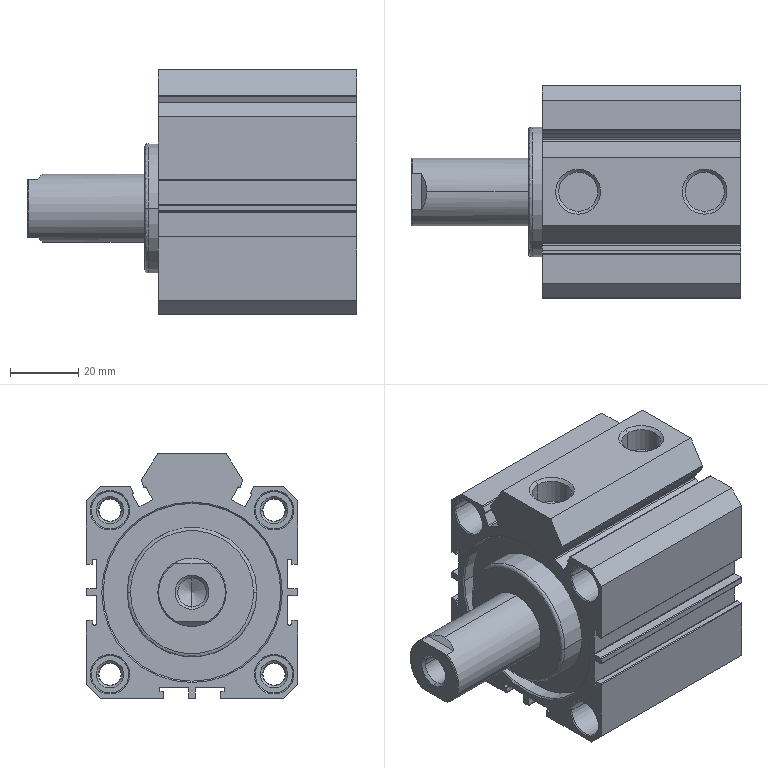Part | SolidWorks | 2 solids | 274 faces | box 96.283 x 62 x 71.5 mm | volume 157551 mm3 | cylinder 116 | plane 94 | cone 62 | spline 2 | commonest cylinder face diameters 0.4 x46 6.647 x16 11 x16 0.8 x10 6.5 x8 11.445 x4